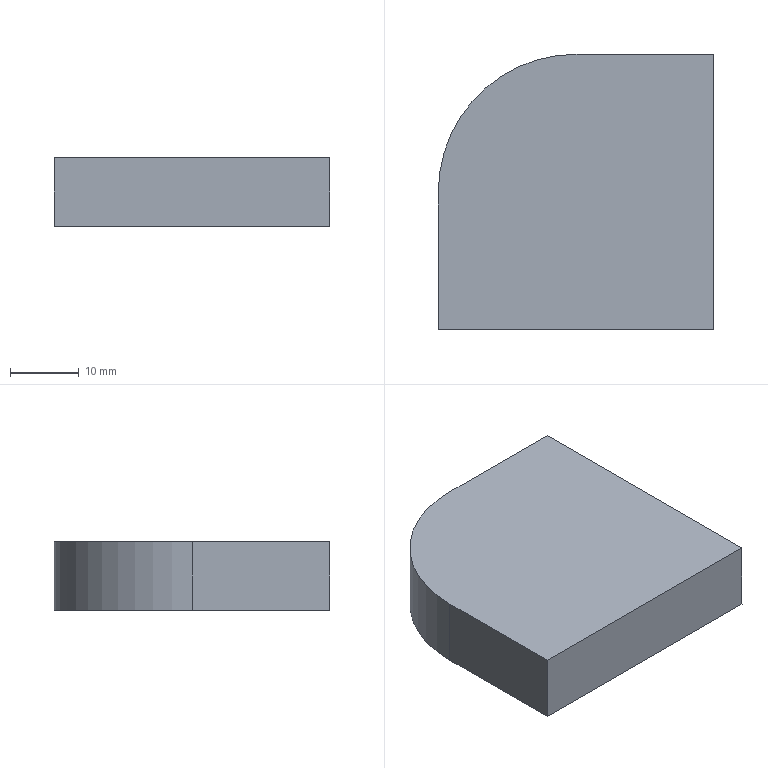Part | SolidWorks | features Extrusion 1, Fillet 1 | 1 solid | 7 faces | box 40 x 40 x 10 mm | volume 15142 mm3 | plane 6 | cylinder 1 | commonest cylinder face diameters 40 x1
STEP:
#1=CARTESIAN_POINT('',(0.,0.,0.));
#2=VERTEX_POINT('',#1);
#3=CARTESIAN_POINT('',(40.,0.,0.));
#4=VERTEX_POINT('',#3);
#5=CARTESIAN_POINT('',(40.,0.,0.));
#6=DIRECTION('',(1.,0.,0.));
#7=VECTOR('',#6,1000.);
#8=LINE('',#5,#7);
#9=EDGE_CURVE('',#2,#4,#8,.T.);
#10=ORIENTED_EDGE('',*,*,#9,.T.);
#11=CARTESIAN_POINT('',(40.,0.,10.));
#12=VERTEX_POINT('',#11);
#13=CARTESIAN_POINT('',(40.,0.,10.));
#14=DIRECTION('',(0.,0.,-1.));
#15=VECTOR('',#14,1000.);
#16=LINE('',#13,#15);
#17=EDGE_CURVE('',#12,#4,#16,.T.);
#18=ORIENTED_EDGE('',*,*,#17,.F.);
#19=CARTESIAN_POINT('',(0.,0.,10.));
#20=VERTEX_POINT('',#19);
#21=CARTESIAN_POINT('',(40.,0.,10.));
#22=DIRECTION('',(1.,0.,0.));
#23=VECTOR('',#22,1000.);
#24=LINE('',#21,#23);
#25=EDGE_CURVE('',#20,#12,#24,.T.);
#26=ORIENTED_EDGE('',*,*,#25,.F.);
#27=CARTESIAN_POINT('',(0.,0.,10.));
#28=DIRECTION('',(0.,0.,-1.));
#29=VECTOR('',#28,1000.);
#30=LINE('',#27,#29);
#31=EDGE_CURVE('',#20,#2,#30,.T.);
#32=ORIENTED_EDGE('',*,*,#31,.T.);
#33=EDGE_LOOP('',(#10,#18,#26,#32));
#34=FACE_OUTER_BOUND('',#33,.T.);
#35=CARTESIAN_POINT('',(40.,0.,10.));
#36=DIRECTION('',(0.,1.,0.));
#37=DIRECTION('',(0.,0.,1.));
#38=AXIS2_PLACEMENT_3D('',#35,#36,#37);
#39=PLANE('',#38);
#40=ADVANCED_FACE('',(#34),#39,.F.);
#41=CARTESIAN_POINT('',(40.,40.,0.));
#42=VERTEX_POINT('',#41);
#43=CARTESIAN_POINT('',(40.,40.,0.));
#44=DIRECTION('',(0.,1.,0.));
#45=VECTOR('',#44,1000.);
#46=LINE('',#43,#45);
#47=EDGE_CURVE('',#4,#42,#46,.T.);
#48=ORIENTED_EDGE('',*,*,#47,.T.);
#49=CARTESIAN_POINT('',(40.,40.,10.));
#50=VERTEX_POINT('',#49);
#51=CARTESIAN_POINT('',(40.,40.,10.));
#52=DIRECTION('',(0.,0.,-1.));
#53=VECTOR('',#52,1000.);
#54=LINE('',#51,#53);
#55=EDGE_CURVE('',#50,#42,#54,.T.);
#56=ORIENTED_EDGE('',*,*,#55,.F.);
#57=CARTESIAN_POINT('',(40.,40.,10.));
#58=DIRECTION('',(0.,1.,0.));
#59=VECTOR('',#58,1000.);
#60=LINE('',#57,#59);
#61=EDGE_CURVE('',#12,#50,#60,.T.);
#62=ORIENTED_EDGE('',*,*,#61,.F.);
#63=ORIENTED_EDGE('',*,*,#17,.T.);
#64=EDGE_LOOP('',(#48,#56,#62,#63));
#65=FACE_OUTER_BOUND('',#64,.T.);
#66=CARTESIAN_POINT('',(40.,40.,10.));
#67=DIRECTION('',(-1.,0.,0.));
#68=DIRECTION('',(0.,0.,1.));
#69=AXIS2_PLACEMENT_3D('',#66,#67,#68);
#70=PLANE('',#69);
#71=ADVANCED_FACE('',(#65),#70,.F.);
#72=CARTESIAN_POINT('',(20.,40.,0.));
#73=VERTEX_POINT('',#72);
#74=CARTESIAN_POINT('',(0.,40.,0.));
#75=DIRECTION('',(-1.,0.,0.));
#76=VECTOR('',#75,1000.);
#77=LINE('',#74,#76);
#78=EDGE_CURVE('',#42,#73,#77,.T.);
#79=ORIENTED_EDGE('',*,*,#78,.T.);
#80=CARTESIAN_POINT('',(20.,40.,10.));
#81=VERTEX_POINT('',#80);
#82=CARTESIAN_POINT('',(20.,40.,10.));
#83=DIRECTION('',(0.,0.,1.));
#84=VECTOR('',#83,1000.);
#85=LINE('',#82,#84);
#86=EDGE_CURVE('',#73,#81,#85,.T.);
#87=ORIENTED_EDGE('',*,*,#86,.T.);
#88=CARTESIAN_POINT('',(0.,40.,10.));
#89=DIRECTION('',(-1.,0.,0.));
#90=VECTOR('',#89,1000.);
#91=LINE('',#88,#90);
#92=EDGE_CURVE('',#50,#81,#91,.T.);
#93=ORIENTED_EDGE('',*,*,#92,.F.);
#94=ORIENTED_EDGE('',*,*,#55,.T.);
#95=EDGE_LOOP('',(#79,#87,#93,#94));
#96=FACE_OUTER_BOUND('',#95,.T.);
#97=CARTESIAN_POINT('',(0.,40.,10.));
#98=DIRECTION('',(0.,-1.,0.));
#99=DIRECTION('',(0.,0.,-1.));
#100=AXIS2_PLACEMENT_3D('',#97,#98,#99);
#101=PLANE('',#100);
#102=ADVANCED_FACE('',(#96),#101,.F.);
#103=CARTESIAN_POINT('',(0.,20.,10.));
#104=VERTEX_POINT('',#103);
#105=CARTESIAN_POINT('',(0.,0.,10.));
#106=DIRECTION('',(0.,-1.,0.));
#107=VECTOR('',#106,1000.);
#108=LINE('',#105,#107);
#109=EDGE_CURVE('',#104,#20,#108,.T.);
#110=ORIENTED_EDGE('',*,*,#109,.F.);
#111=CARTESIAN_POINT('',(0.,20.,0.));
#112=VERTEX_POINT('',#111);
#113=CARTESIAN_POINT('',(0.,20.,10.));
#114=DIRECTION('',(0.,0.,-1.));
#115=VECTOR('',#114,1000.);
#116=LINE('',#113,#115);
#117=EDGE_CURVE('',#104,#112,#116,.T.);
#118=ORIENTED_EDGE('',*,*,#117,.T.);
#119=CARTESIAN_POINT('',(0.,0.,0.));
#120=DIRECTION('',(0.,-1.,0.));
#121=VECTOR('',#120,1000.);
#122=LINE('',#119,#121);
#123=EDGE_CURVE('',#112,#2,#122,.T.);
#124=ORIENTED_EDGE('',*,*,#123,.T.);
#125=ORIENTED_EDGE('',*,*,#31,.F.);
#126=EDGE_LOOP('',(#110,#118,#124,#125));
#127=FACE_OUTER_BOUND('',#126,.T.);
#128=CARTESIAN_POINT('',(0.,0.,10.));
#129=DIRECTION('',(1.,0.,0.));
#130=DIRECTION('',(0.,0.,-1.));
#131=AXIS2_PLACEMENT_3D('',#128,#129,#130);
#132=PLANE('',#131);
#133=ADVANCED_FACE('',(#127),#132,.F.);
#134=ORIENTED_EDGE('',*,*,#92,.T.);
#135=CARTESIAN_POINT('',(20.,20.,10.));
#136=DIRECTION('',(0.,0.,1.));
#137=DIRECTION('',(-1.,0.,0.));
#138=AXIS2_PLACEMENT_3D('',#135,#136,#137);
#139=CIRCLE('',#138,20.);
#140=EDGE_CURVE('',#81,#104,#139,.T.);
#141=ORIENTED_EDGE('',*,*,#140,.T.);
#142=ORIENTED_EDGE('',*,*,#109,.T.);
#143=ORIENTED_EDGE('',*,*,#25,.T.);
#144=ORIENTED_EDGE('',*,*,#61,.T.);
#145=EDGE_LOOP('',(#134,#141,#142,#143,#144));
#146=FACE_OUTER_BOUND('',#145,.T.);
#147=CARTESIAN_POINT('',(0.,0.,10.));
#148=DIRECTION('',(0.,0.,-1.));
#149=DIRECTION('',(-1.,0.,0.));
#150=AXIS2_PLACEMENT_3D('',#147,#148,#149);
#151=PLANE('',#150);
#152=ADVANCED_FACE('',(#146),#151,.F.);
#153=ORIENTED_EDGE('',*,*,#123,.F.);
#154=CARTESIAN_POINT('',(20.,20.,0.));
#155=DIRECTION('',(0.,0.,-1.));
#156=DIRECTION('',(-1.,0.,0.));
#157=AXIS2_PLACEMENT_3D('',#154,#155,#156);
#158=CIRCLE('',#157,20.);
#159=EDGE_CURVE('',#112,#73,#158,.T.);
#160=ORIENTED_EDGE('',*,*,#159,.T.);
#161=ORIENTED_EDGE('',*,*,#78,.F.);
#162=ORIENTED_EDGE('',*,*,#47,.F.);
#163=ORIENTED_EDGE('',*,*,#9,.F.);
#164=EDGE_LOOP('',(#153,#160,#161,#162,#163));
#165=FACE_OUTER_BOUND('',#164,.T.);
#166=CARTESIAN_POINT('',(0.,0.,0.));
#167=DIRECTION('',(0.,0.,-1.));
#168=DIRECTION('',(-1.,0.,0.));
#169=AXIS2_PLACEMENT_3D('',#166,#167,#168);
#170=PLANE('',#169);
#171=ADVANCED_FACE('',(#165),#170,.T.);
#172=ORIENTED_EDGE('',*,*,#140,.F.);
#173=ORIENTED_EDGE('',*,*,#86,.F.);
#174=ORIENTED_EDGE('',*,*,#159,.F.);
#175=ORIENTED_EDGE('',*,*,#117,.F.);
#176=EDGE_LOOP('',(#172,#173,#174,#175));
#177=FACE_OUTER_BOUND('',#176,.T.);
#178=CARTESIAN_POINT('',(20.,20.,10.));
#179=DIRECTION('',(0.,0.,-1.));
#180=DIRECTION('',(-1.,0.,0.));
#181=AXIS2_PLACEMENT_3D('',#178,#179,#180);
#182=CYLINDRICAL_SURFACE('',#181,20.);
#183=ADVANCED_FACE('',(#177),#182,.T.);
#184=CLOSED_SHELL('',(#40,#71,#102,#133,#152,#171,#183));
#185=MANIFOLD_SOLID_BREP('',#184);
#186=CARTESIAN_POINT('',(0.,0.,0.));
#187=DIRECTION('',(0.,0.,1.));
#188=DIRECTION('',(1.,0.,0.));
#189=AXIS2_PLACEMENT_3D('',#186,#187,#188);
#190=(LENGTH_UNIT()NAMED_UNIT(*)SI_UNIT(.MILLI.,.METRE.));
#191=UNCERTAINTY_MEASURE_WITH_UNIT(LENGTH_MEASURE(0.00001),#190,'','');
#192=(NAMED_UNIT(*)PLANE_ANGLE_UNIT()SI_UNIT($,.RADIAN.));
#193=(NAMED_UNIT(*)SI_UNIT($,.STERADIAN.)SOLID_ANGLE_UNIT());
#194=(GEOMETRIC_REPRESENTATION_CONTEXT(3)GLOBAL_UNCERTAINTY_ASSIGNED_CONTEXT((#191))GLOBAL_UNIT_ASSIGNED_CONTEXT((#190,#192,#193))REPRESENTATION_CONTEXT('',''));
#195=ADVANCED_BREP_SHAPE_REPRESENTATION('',(#185,#189),#194);